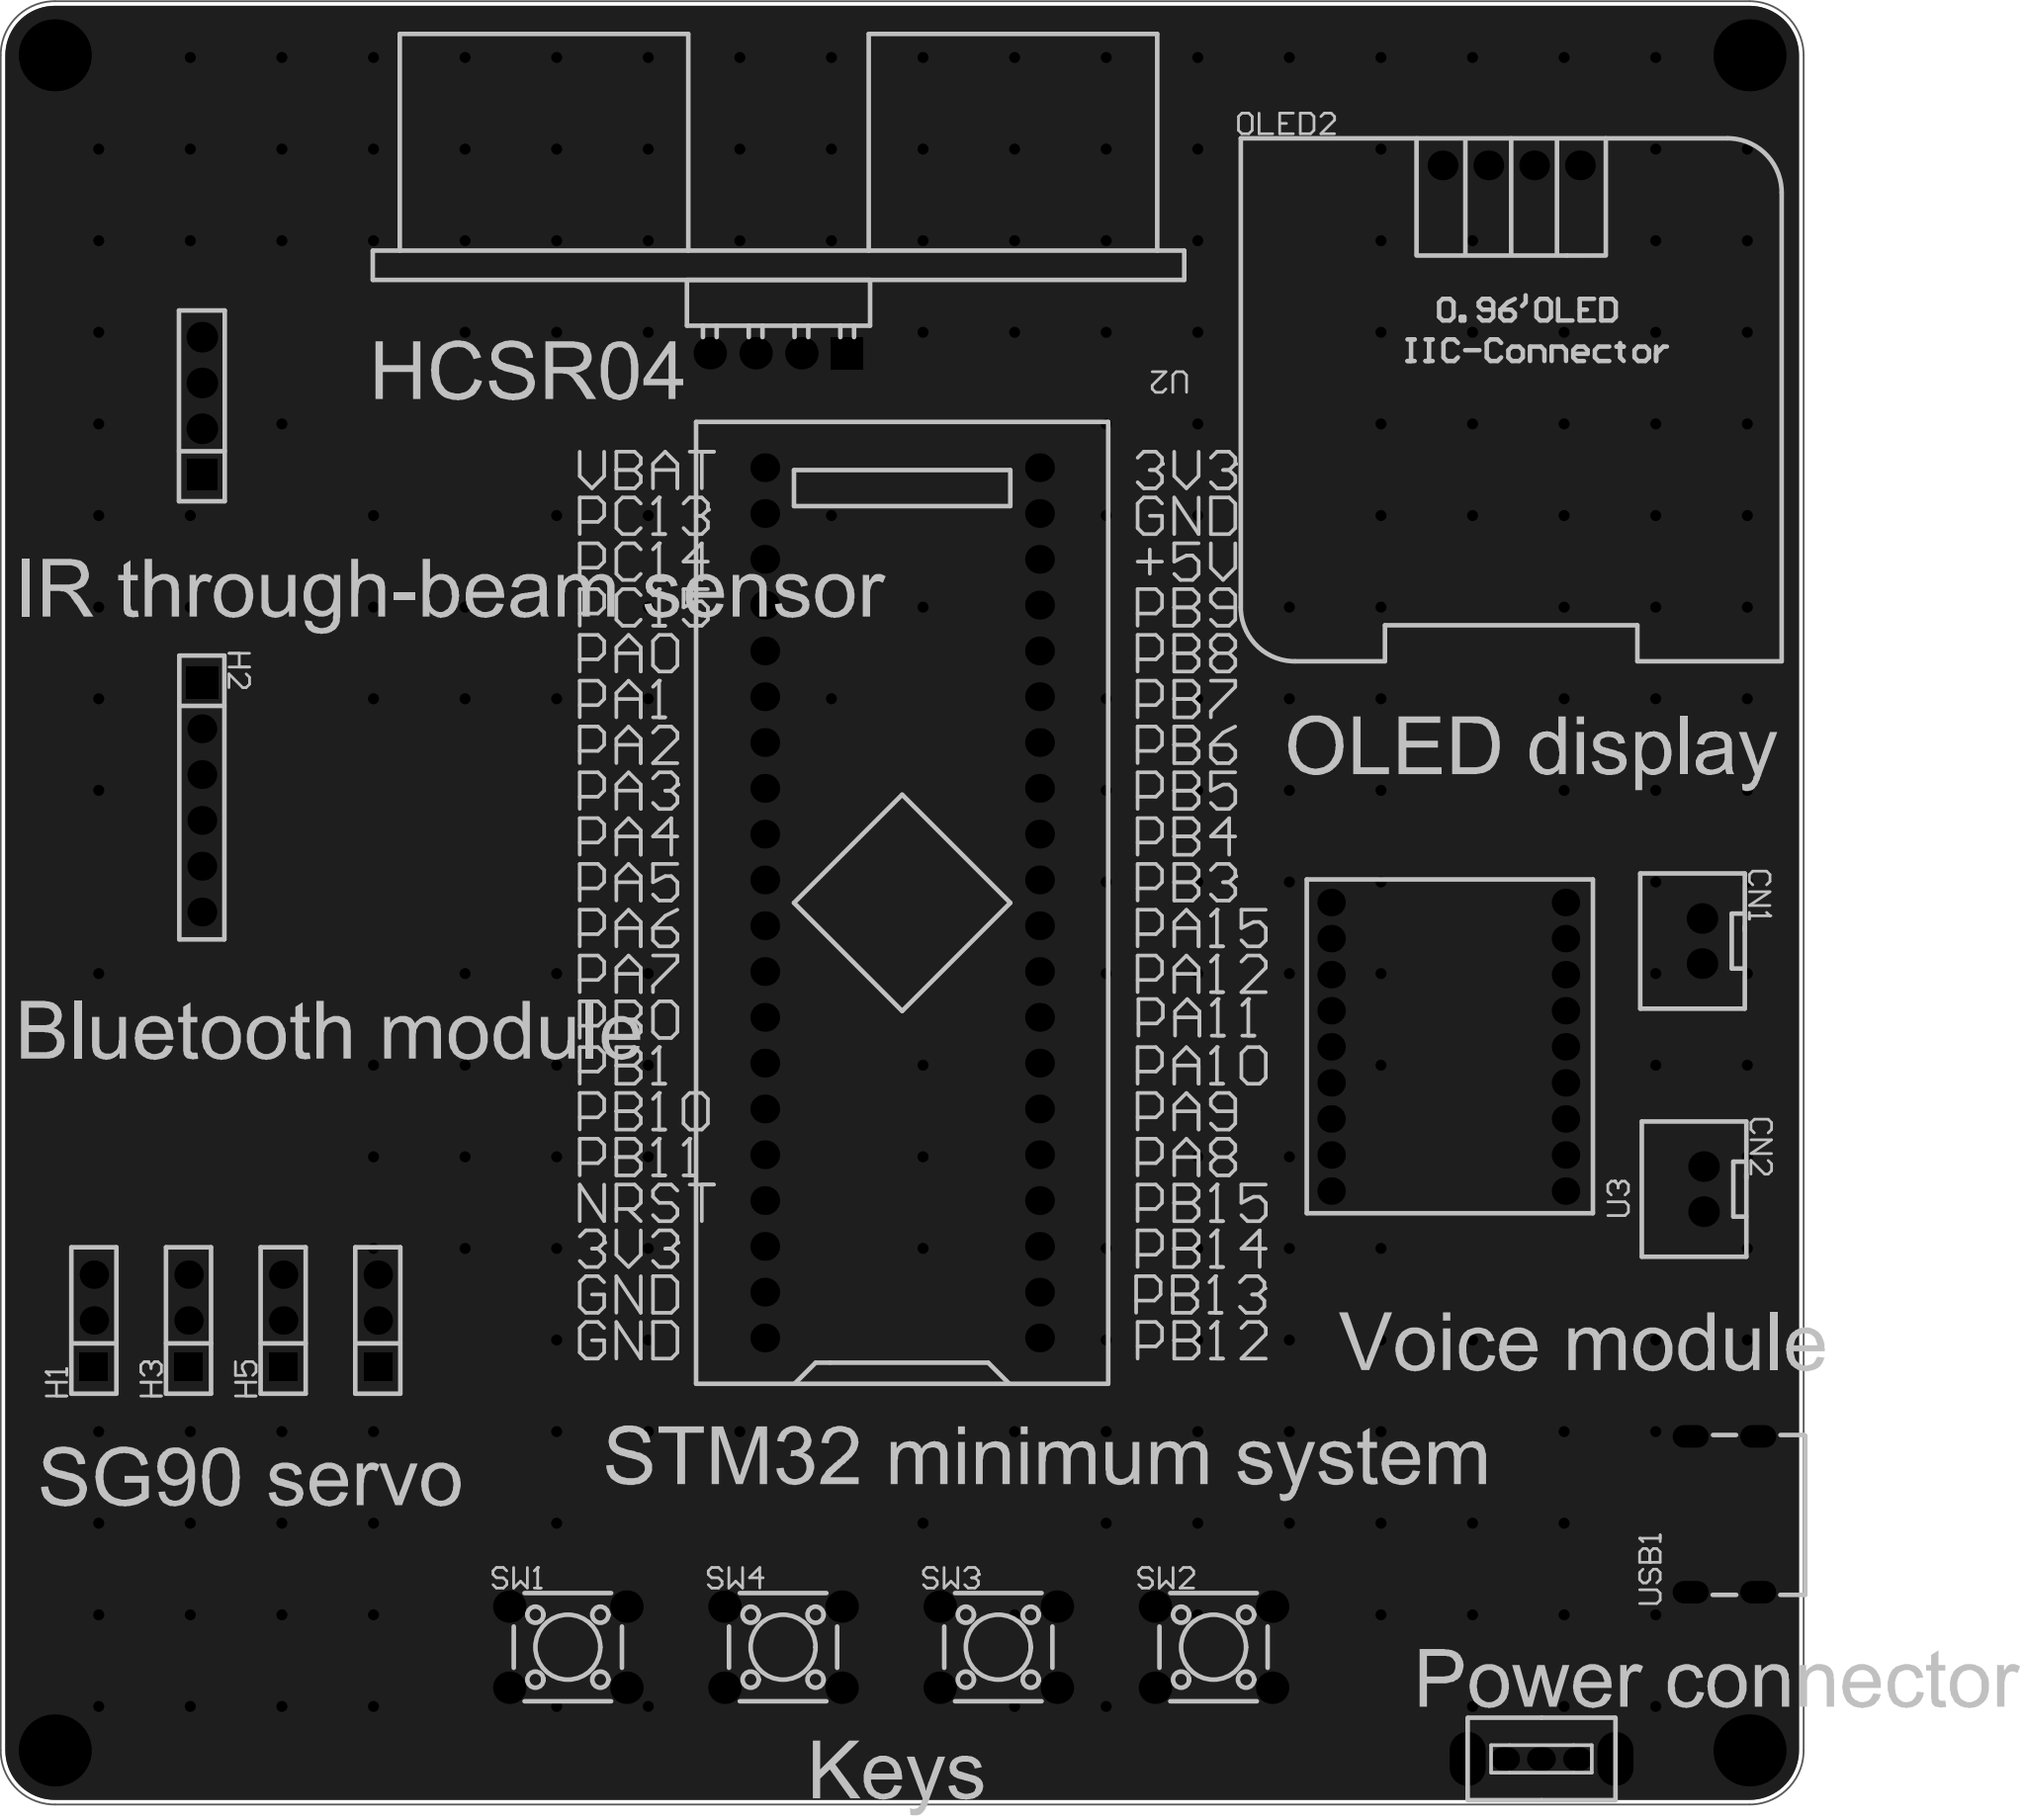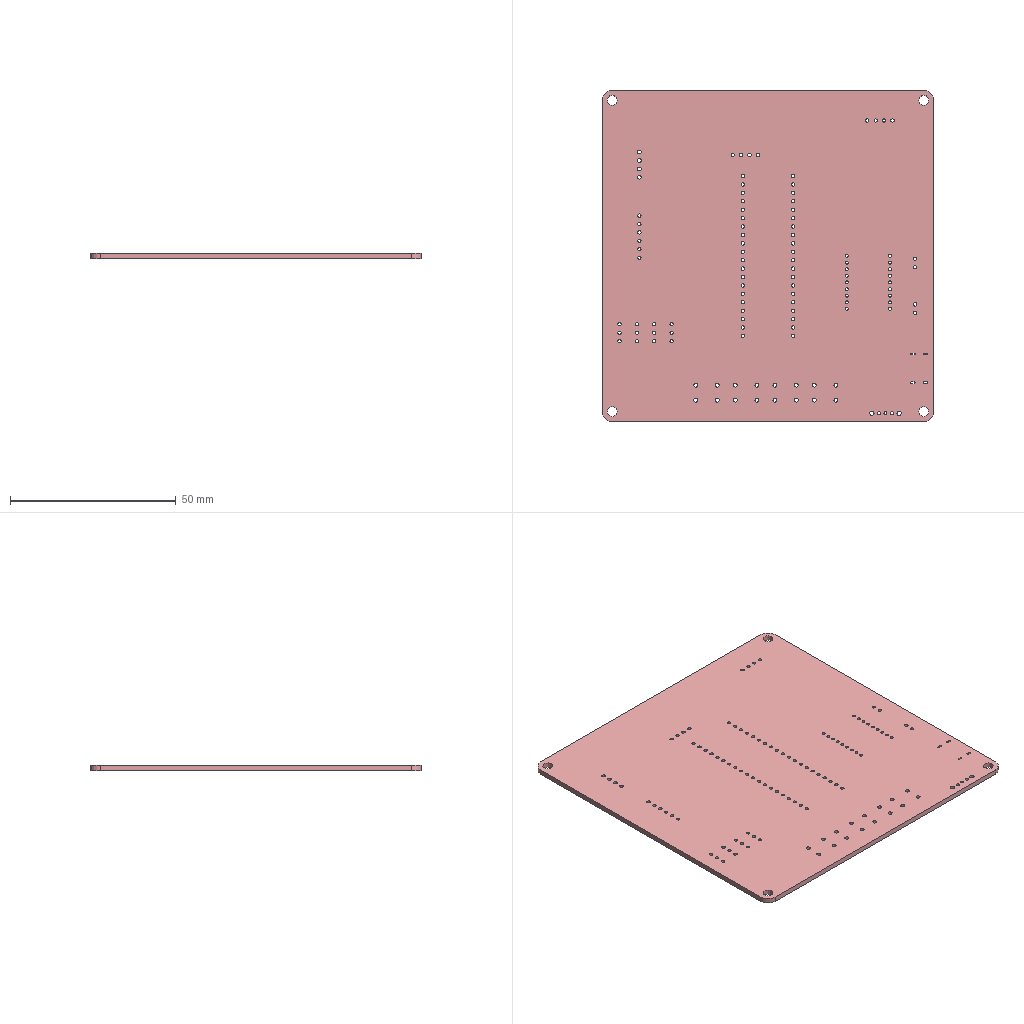Circuit board layout | Altium Designer | box 100 x 100 x 1.6 mm
Layer stack:
# Altium Designer layer stack of  (unit mm; dielectric type: 0 none, 1 core, 2 prepreg, 3 surface material)
index,name,kind,layer,copper_thickness_mm,dielectric_type,dielectric_thickness_mm,dielectric_material,dielectric_constant
0,Top Paste Mask Layer,other,,,,,,
1,Top Silkscreen Layer,other,,,,,,
2,Top Solder Mask Layer,dielectric,,,3,0.01,,3.3
3,Top Layer,copper,Top Layer,0.035,,,,
4,Dielectric1,dielectric,,,3,1.51,FR4,4.5
5,Bottom Layer,copper,Bottom Layer,0.035,,,,
6,Bottom Solder Mask Layer,dielectric,,,3,0.01,,3.3
7,Bottom Silkscreen Layer,other,,,,,,
8,Bottom Paste Mask Layer,other,,,,,,
# drill layer pairs: low layer,high layer
drill_pair,Top Layer,Bottom Layer
Part placement:
Designator,Comment,Layer,Footprint,Center-X(mm),Center-Y(mm),Rotation
U1,STM32F103C8T6-Card,TopLayer,CONN-TH_L53.3-W22.9_STM32F103C8T6-CARD,141.351,130.937,90
SW1,,TopLayer,SW-TH_4P-L6.0-W6.0-P4.50-LS6.5,122.809,89.662,0
SW2,,TopLayer,SW-TH_4P-L6.0-W6.0-P4.50-LS6.5,158.623,89.662,0
SW3,,TopLayer,SW-TH_4P-L6.0-W6.0-P4.50-LS6.5,146.685,89.662,0
SW4,,TopLayer,SW-TH_4P-L6.0-W6.0-P4.50-LS6.5,134.747,89.662,0
H12,,TopLayer,HDR-TH_3P-P2.54-V-F,112.268,107.778,90
SW5,,TopLayer,拨动开关,176.817,83.464,0
H4,,TopLayer,HDR-TH_4P-P2.54-V-F,102.509,158.496,90
H2,,TopLayer,HDR-TH_6P-P2.54-V-F,102.509,136.779,270
OLED2,,TopLayer,0.96OLED_4P,175.133,171.831,0
CN1,XH2.54*2P_THT,TopLayer,CONN-TH_2P-P2.50-XH2.54-2P,185.714,128.818,270
CN2,XH2.54*2P_THT,TopLayer,CONN-TH_2P-P2.50-XH2.54-2P,185.801,115.062,270
U2,HC-SR04,TopLayer,TH_HC-SR04V,134.493,161.417,180
U3,CON2.0MM-PAD-18,TopLayer,CONN-TH_18P-P2.00_C9900078766,171.644,122.954,90
USB1,,TopLayer,USB__TYPE-C-6P,186.696,97.03,90
H1,,TopLayer,HDR-TH_3P-P2.54-V-F,96.52,107.778,90
H3,,TopLayer,HDR-TH_3P-P2.54-V-F,101.769,107.778,90
H5,,TopLayer,HDR-TH_3P-P2.54-V-F,107.019,107.778,90
Pad and via stacks:
# Altium Designer via and pad stacks of  (unit mm). Each distinct definition once, with the count of objects using it.
# via: kind,start_layer,end_layer,hole_mm,diameter_mm,mode(0 simple;1 top-mid-bottom;2 full stack),diameter_per_layer,count,example_net
# pad: kind,layer,hole_mm,hole_type(0 round;1 square;2 slot),plating,top_size,top_shape(1 round;2 rect;3 octagon;9 rounded rect),mid_size,bottom_size,mode,footprint,size_per_layer,count,example
pad,Multi-Layer,3,0,plated,4x4,1,4x4,4x4,0,,,4,1
pad,Multi-Layer,1,0,plated,1.6x1.6,1,1.6x1.6,1.6x1.6,0,CONN-TH_L53.3-W22.9_STM32F103C8T6-CARD,,40,U1.1
pad,Multi-Layer,1.2,0,plated,1.8x1.8,1,1.8x1.8,1.8x1.8,0,SW-TH_4P-L6.0-W6.0-P4.50-LS6.5,,16,SW1.1
pad,Multi-Layer,1.02,0,plated,1.575x1.575,1,1.575x1.575,1.575x1.575,0,HDR-TH_3P-P2.54-V-F,,8,H12.3
pad,Multi-Layer,1.02,0,plated,1.575x1.575,2,1.575x1.575,1.575x1.575,0,HDR-TH_3P-P2.54-V-F,,4,H12.1
pad,Multi-Layer,0.8992,0,plated,1.6x1.3,1,1.6x1.3,1.6x1.3,0,\u00B2\u00A6\u00B6\u00AF\u00BF\u00AA\u00B9\u00D8,,3,SW5.1
pad,Multi-Layer,1.3,0,plated,3x1.999,1,3x1.999,3x1.999,0,\u00B2\u00A6\u00B6\u00AF\u00BF\u00AA\u00B9\u00D8,,2,SW5.4
pad,Multi-Layer,1.1,0,plated,1.7x1.7,2,1.7x1.7,1.7x1.7,0,HDR-TH_4P-P2.54-V-F,,1,H4.1
pad,Multi-Layer,1.1,0,plated,1.7x1.7,1,1.7x1.7,1.7x1.7,0,HDR-TH_4P-P2.54-V-F,,3,H4.2
pad,Multi-Layer,1.02,0,plated,1.6x1.6,1,1.6x1.6,1.6x1.6,0,HDR-TH_6P-P2.54-V-F,,5,H2.6
pad,Multi-Layer,1.02,0,plated,1.8x1.8,2,1.8x1.8,1.8x1.8,0,HDR-TH_6P-P2.54-V-F,,1,H2.1
pad,Multi-Layer,1,0,plated,1.65x1.65,1,1.65x1.65,1.65x1.65,0,0.96OLED_4P,,4,OLED2.4
pad,Multi-Layer,1.05,0,plated,1.7x1.7,1,1.7x1.7,1.7x1.7,0,CONN-TH_2P-P2.50-XH2.54-2P,,4,CN1.2
pad,Multi-Layer,1.001,0,plated,1.8x1.8,1,1.8x1.8,1.8x1.8,0,TH_HC-SR04V,,3,U2.4
pad,Multi-Layer,1.001,0,plated,1.8x1.8,2,1.8x1.8,1.8x1.8,0,TH_HC-SR04V,,1,U2.1
pad,Multi-Layer,0.9,0,plated,1.524x1.524,1,1.524x1.524,1.524x1.524,0,CONN-TH_18P-P2.00_C9900078766,,18,U3.1
pad,Multi-Layer,0.6,2,plated,1.25x2,1,1.25x2,1.25x2,0,USB_ TYPE-C-6P,,4,USB1.8
pad,Top Layer,0,0,plated,0.7x1.2,2,0.7x1.2,0.7x1.2,0,USB_ TYPE-C-6P,,2,USB1.A5
pad,Top Layer,0,0,plated,0.8x1.2,2,0.8x1.2,0.8x1.2,0,USB_ TYPE-C-6P,,2,USB1.B9
pad,Top Layer,0,0,plated,0.9x1.2,2,0.9x1.2,0.9x1.2,0,USB_ TYPE-C-6P,,2,USB1.B12
via,Top Layer,Bottom Layer,0.3048,0.61,0,,215,GND
Copper pours:
name,layer,net,type(0 solid;1 hatched;2 none)
Bottom Layer-GND,Bottom Layer,GND,0
Top Layer-GND,Top Layer,GND,0
Design rules, without the lines most boards share:
# Altium Designer design rules of  (exported by Altium Designer, unit mm)
# columns: name | kind | enabled | priority | scope1 | scope2 | descriptor | typed fields (field=value)
Copper_copperRegion_copperThickness1oz | 0 | disabled | 4 | All | All | Clearance Constraint (Gap=5.984mil) (Disabled)(All),(All) | gap=0.152
Copper_copperRegion_copperThickness1oz_1 | 63 | disabled | 4 | All | All | Board Clearance Constraint (Gap=0mil) (Disabled)(All) |
Copper_copperRegion_Copper_copperRegion | 0 | disabled | 5 | All | All | Clearance Constraint (Gap=5.984mil) (Disabled)(All),(All) | gap=0.152
Copper_copperRegion_Copper_copperRegion_1 | 63 | disabled | 5 | All | All | Board Clearance Constraint (Gap=0mil) (Disabled)(All) |
copperThickness1oz | 0 | enabled | 6 | All | All | Clearance Constraint (Gap=5.984mil) (All),(All) | gap=0.152
copperThickness1oz_1 | 63 | enabled | 6 | All | All | Board Clearance Constraint (Gap=0mil) (All) |
copperRegion_copperThickness1oz | 20 | disabled | 1 | All | All | Polygon Connect Rule(Relief Connect )(Conductor Width=10mil) (Relief Angle=90 Angle) (Entries=4) (Air Gap Width=10mil) (Disabled)(All),(All) | connect_style(0=relief,1=direct,2=none)=0 relief_conductor_width=0.254 relief_entries=4
copperRegion_Copper_copperRegion | 20 | disabled | 2 | All | All | Polygon Connect Rule(Relief Connect )(Conductor Width=10mil) (Relief Angle=90 Angle) (Entries=4) (Air Gap Width=10mil) (Disabled)(All),(All) | connect_style(0=relief,1=direct,2=none)=0 relief_conductor_width=0.254 relief_entries=4
copperRegion | 20 | enabled | 3 | All | All | Polygon Connect Rule(Relief Connect )(Conductor Width=10mil) (Relief Angle=90 Angle) (Entries=4) (Air Gap Width=10mil) (All),(All) | connect_style(0=relief,1=direct,2=none)=0 relief_conductor_width=0.254 relief_entries=4